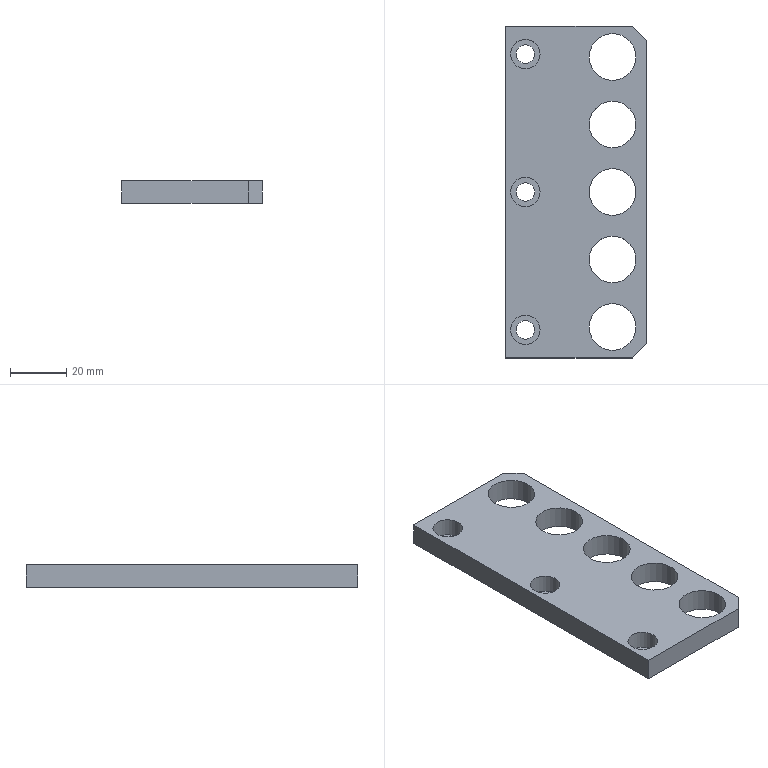Part | NX | 1 solid | 22 faces | box 50 x 118 x 8 mm | volume 36501 mm3 | cylinder 11 | plane 11 | commonest cylinder face diameters 16.6 x5 6.6 x3 10.5 x3
STEP:
#1=CARTESIAN_POINT('',(-14.7,49.,-8.));
#2=VERTEX_POINT('',#1);
#3=CARTESIAN_POINT('',(-18.,49.,-8.));
#4=DIRECTION('',(0.,0.,1.));
#5=DIRECTION('',(1.,0.,0.));
#6=AXIS2_PLACEMENT_3D('',#3,#4,#5);
#7=CIRCLE('',#6,3.3);
#8=EDGE_CURVE('',#2,#2,#7,.F.);
#9=ORIENTED_EDGE('',*,*,#8,.T.);
#10=EDGE_LOOP('',(#9));
#11=FACE_BOUND('',#10,.T.);
#12=CARTESIAN_POINT('',(-14.7,49.,-6.5));
#13=VERTEX_POINT('',#12);
#14=CARTESIAN_POINT('',(-18.,49.,-6.5));
#15=DIRECTION('',(0.,0.,1.));
#16=DIRECTION('',(1.,0.,0.));
#17=AXIS2_PLACEMENT_3D('',#14,#15,#16);
#18=CIRCLE('',#17,3.3);
#19=EDGE_CURVE('',#13,#13,#18,.F.);
#20=ORIENTED_EDGE('',*,*,#19,.F.);
#21=EDGE_LOOP('',(#20));
#22=FACE_BOUND('',#21,.T.);
#23=CARTESIAN_POINT('',(-18.,49.,-8.));
#24=DIRECTION('',(0.,0.,1.));
#25=DIRECTION('',(1.,0.,0.));
#26=AXIS2_PLACEMENT_3D('',#23,#24,#25);
#27=CYLINDRICAL_SURFACE('',#26,3.3);
#28=ADVANCED_FACE('',(#11,#22),#27,.F.);
#29=CARTESIAN_POINT('',(21.3,48.,0.));
#30=VERTEX_POINT('',#29);
#31=CARTESIAN_POINT('',(13.,48.,0.));
#32=DIRECTION('',(0.,0.,1.));
#33=DIRECTION('',(1.,0.,0.));
#34=AXIS2_PLACEMENT_3D('',#31,#32,#33);
#35=CIRCLE('',#34,8.3);
#36=EDGE_CURVE('',#30,#30,#35,.F.);
#37=ORIENTED_EDGE('',*,*,#36,.T.);
#38=EDGE_LOOP('',(#37));
#39=FACE_BOUND('',#38,.T.);
#40=CARTESIAN_POINT('',(21.3,24.,0.));
#41=VERTEX_POINT('',#40);
#42=CARTESIAN_POINT('',(13.,24.,0.));
#43=DIRECTION('',(0.,0.,1.));
#44=DIRECTION('',(1.,0.,0.));
#45=AXIS2_PLACEMENT_3D('',#42,#43,#44);
#46=CIRCLE('',#45,8.3);
#47=EDGE_CURVE('',#41,#41,#46,.F.);
#48=ORIENTED_EDGE('',*,*,#47,.T.);
#49=EDGE_LOOP('',(#48));
#50=FACE_BOUND('',#49,.T.);
#51=CARTESIAN_POINT('',(21.3,0.,0.));
#52=VERTEX_POINT('',#51);
#53=CARTESIAN_POINT('',(13.,0.,0.));
#54=DIRECTION('',(0.,0.,1.));
#55=DIRECTION('',(1.,0.,0.));
#56=AXIS2_PLACEMENT_3D('',#53,#54,#55);
#57=CIRCLE('',#56,8.3);
#58=EDGE_CURVE('',#52,#52,#57,.F.);
#59=ORIENTED_EDGE('',*,*,#58,.T.);
#60=EDGE_LOOP('',(#59));
#61=FACE_BOUND('',#60,.T.);
#62=CARTESIAN_POINT('',(21.3,-24.,0.));
#63=VERTEX_POINT('',#62);
#64=CARTESIAN_POINT('',(13.,-24.,0.));
#65=DIRECTION('',(0.,0.,1.));
#66=DIRECTION('',(1.,0.,0.));
#67=AXIS2_PLACEMENT_3D('',#64,#65,#66);
#68=CIRCLE('',#67,8.3);
#69=EDGE_CURVE('',#63,#63,#68,.F.);
#70=ORIENTED_EDGE('',*,*,#69,.T.);
#71=EDGE_LOOP('',(#70));
#72=FACE_BOUND('',#71,.T.);
#73=CARTESIAN_POINT('',(21.3,-48.,0.));
#74=VERTEX_POINT('',#73);
#75=CARTESIAN_POINT('',(13.,-48.,0.));
#76=DIRECTION('',(0.,0.,1.));
#77=DIRECTION('',(1.,0.,0.));
#78=AXIS2_PLACEMENT_3D('',#75,#76,#77);
#79=CIRCLE('',#78,8.3);
#80=EDGE_CURVE('',#74,#74,#79,.F.);
#81=ORIENTED_EDGE('',*,*,#80,.T.);
#82=EDGE_LOOP('',(#81));
#83=FACE_BOUND('',#82,.T.);
#84=CARTESIAN_POINT('',(-25.,-59.,0.));
#85=VERTEX_POINT('',#84);
#86=CARTESIAN_POINT('',(-25.,59.,0.));
#87=VERTEX_POINT('',#86);
#88=CARTESIAN_POINT('',(-25.,59.,0.));
#89=DIRECTION('',(0.,-1.,0.));
#90=VECTOR('',#89,1000.);
#91=LINE('',#88,#90);
#92=EDGE_CURVE('',#85,#87,#91,.F.);
#93=ORIENTED_EDGE('',*,*,#92,.F.);
#94=CARTESIAN_POINT('',(20.,-59.,0.));
#95=VERTEX_POINT('',#94);
#96=CARTESIAN_POINT('',(-25.,-59.,0.));
#97=DIRECTION('',(1.,0.,0.));
#98=VECTOR('',#97,1000.);
#99=LINE('',#96,#98);
#100=EDGE_CURVE('',#95,#85,#99,.F.);
#101=ORIENTED_EDGE('',*,*,#100,.F.);
#102=CARTESIAN_POINT('',(25.,-54.,0.));
#103=VERTEX_POINT('',#102);
#104=CARTESIAN_POINT('',(20.,-59.,0.));
#105=DIRECTION('',(0.7071,0.7071,0.));
#106=VECTOR('',#105,1000.);
#107=LINE('',#104,#106);
#108=EDGE_CURVE('',#103,#95,#107,.F.);
#109=ORIENTED_EDGE('',*,*,#108,.F.);
#110=CARTESIAN_POINT('',(25.,54.,0.));
#111=VERTEX_POINT('',#110);
#112=CARTESIAN_POINT('',(25.,-54.,0.));
#113=DIRECTION('',(0.,1.,0.));
#114=VECTOR('',#113,1000.);
#115=LINE('',#112,#114);
#116=EDGE_CURVE('',#111,#103,#115,.F.);
#117=ORIENTED_EDGE('',*,*,#116,.F.);
#118=CARTESIAN_POINT('',(20.,59.,0.));
#119=VERTEX_POINT('',#118);
#120=CARTESIAN_POINT('',(25.,54.,0.));
#121=DIRECTION('',(-0.7071,0.7071,0.));
#122=VECTOR('',#121,1000.);
#123=LINE('',#120,#122);
#124=EDGE_CURVE('',#119,#111,#123,.F.);
#125=ORIENTED_EDGE('',*,*,#124,.F.);
#126=CARTESIAN_POINT('',(20.,59.,0.));
#127=DIRECTION('',(-1.,0.,0.));
#128=VECTOR('',#127,1000.);
#129=LINE('',#126,#128);
#130=EDGE_CURVE('',#87,#119,#129,.F.);
#131=ORIENTED_EDGE('',*,*,#130,.F.);
#132=EDGE_LOOP('',(#93,#101,#109,#117,#125,#131));
#133=FACE_BOUND('',#132,.T.);
#134=CARTESIAN_POINT('',(-23.25,0.,0.));
#135=VERTEX_POINT('',#134);
#136=CARTESIAN_POINT('',(-18.,0.,0.));
#137=DIRECTION('',(0.,0.,-1.));
#138=DIRECTION('',(-1.,0.,0.));
#139=AXIS2_PLACEMENT_3D('',#136,#137,#138);
#140=CIRCLE('',#139,5.25);
#141=EDGE_CURVE('',#135,#135,#140,.T.);
#142=ORIENTED_EDGE('',*,*,#141,.T.);
#143=EDGE_LOOP('',(#142));
#144=FACE_BOUND('',#143,.T.);
#145=CARTESIAN_POINT('',(-23.25,-49.,0.));
#146=VERTEX_POINT('',#145);
#147=CARTESIAN_POINT('',(-18.,-49.,0.));
#148=DIRECTION('',(0.,0.,-1.));
#149=DIRECTION('',(-1.,0.,0.));
#150=AXIS2_PLACEMENT_3D('',#147,#148,#149);
#151=CIRCLE('',#150,5.25);
#152=EDGE_CURVE('',#146,#146,#151,.T.);
#153=ORIENTED_EDGE('',*,*,#152,.T.);
#154=EDGE_LOOP('',(#153));
#155=FACE_BOUND('',#154,.T.);
#156=CARTESIAN_POINT('',(-12.75,49.,0.));
#157=VERTEX_POINT('',#156);
#158=CARTESIAN_POINT('',(-18.,49.,0.));
#159=DIRECTION('',(0.,0.,1.));
#160=DIRECTION('',(1.,0.,0.));
#161=AXIS2_PLACEMENT_3D('',#158,#159,#160);
#162=CIRCLE('',#161,5.25);
#163=EDGE_CURVE('',#157,#157,#162,.T.);
#164=ORIENTED_EDGE('',*,*,#163,.F.);
#165=EDGE_LOOP('',(#164));
#166=FACE_BOUND('',#165,.T.);
#167=CARTESIAN_POINT('',(-18.,-49.,0.));
#168=DIRECTION('',(0.,0.,1.));
#169=DIRECTION('',(1.,0.,0.));
#170=AXIS2_PLACEMENT_3D('',#167,#168,#169);
#171=PLANE('',#170);
#172=ADVANCED_FACE('',(#39,#50,#61,#72,#83,#133,#144,#155,#166),#171,.T.);
#173=ORIENTED_EDGE('',*,*,#92,.T.);
#174=CARTESIAN_POINT('',(-25.,59.,-8.));
#175=VERTEX_POINT('',#174);
#176=CARTESIAN_POINT('',(-25.,59.,-8.));
#177=DIRECTION('',(0.,0.,1.));
#178=VECTOR('',#177,1000.);
#179=LINE('',#176,#178);
#180=EDGE_CURVE('',#87,#175,#179,.F.);
#181=ORIENTED_EDGE('',*,*,#180,.T.);
#182=CARTESIAN_POINT('',(-25.,-59.,-8.));
#183=VERTEX_POINT('',#182);
#184=CARTESIAN_POINT('',(-25.,59.,-8.));
#185=DIRECTION('',(0.,-1.,0.));
#186=VECTOR('',#185,1000.);
#187=LINE('',#184,#186);
#188=EDGE_CURVE('',#183,#175,#187,.F.);
#189=ORIENTED_EDGE('',*,*,#188,.F.);
#190=CARTESIAN_POINT('',(-25.,-59.,-8.));
#191=DIRECTION('',(0.,0.,1.));
#192=VECTOR('',#191,1000.);
#193=LINE('',#190,#192);
#194=EDGE_CURVE('',#85,#183,#193,.F.);
#195=ORIENTED_EDGE('',*,*,#194,.F.);
#196=EDGE_LOOP('',(#173,#181,#189,#195));
#197=FACE_BOUND('',#196,.T.);
#198=CARTESIAN_POINT('',(-25.,59.,-8.));
#199=DIRECTION('',(-1.,0.,0.));
#200=DIRECTION('',(0.,0.,1.));
#201=AXIS2_PLACEMENT_3D('',#198,#199,#200);
#202=PLANE('',#201);
#203=ADVANCED_FACE('',(#197),#202,.T.);
#204=ORIENTED_EDGE('',*,*,#100,.T.);
#205=ORIENTED_EDGE('',*,*,#194,.T.);
#206=CARTESIAN_POINT('',(20.,-59.,-8.));
#207=VERTEX_POINT('',#206);
#208=CARTESIAN_POINT('',(-25.,-59.,-8.));
#209=DIRECTION('',(1.,0.,0.));
#210=VECTOR('',#209,1000.);
#211=LINE('',#208,#210);
#212=EDGE_CURVE('',#207,#183,#211,.F.);
#213=ORIENTED_EDGE('',*,*,#212,.F.);
#214=CARTESIAN_POINT('',(20.,-59.,-8.));
#215=DIRECTION('',(0.,0.,1.));
#216=VECTOR('',#215,1000.);
#217=LINE('',#214,#216);
#218=EDGE_CURVE('',#95,#207,#217,.F.);
#219=ORIENTED_EDGE('',*,*,#218,.F.);
#220=EDGE_LOOP('',(#204,#205,#213,#219));
#221=FACE_BOUND('',#220,.T.);
#222=CARTESIAN_POINT('',(-25.,-59.,-8.));
#223=DIRECTION('',(0.,-1.,0.));
#224=DIRECTION('',(0.,0.,-1.));
#225=AXIS2_PLACEMENT_3D('',#222,#223,#224);
#226=PLANE('',#225);
#227=ADVANCED_FACE('',(#221),#226,.T.);
#228=ORIENTED_EDGE('',*,*,#108,.T.);
#229=ORIENTED_EDGE('',*,*,#218,.T.);
#230=CARTESIAN_POINT('',(25.,-54.,-8.));
#231=VERTEX_POINT('',#230);
#232=CARTESIAN_POINT('',(20.,-59.,-8.));
#233=DIRECTION('',(0.7071,0.7071,0.));
#234=VECTOR('',#233,1000.);
#235=LINE('',#232,#234);
#236=EDGE_CURVE('',#231,#207,#235,.F.);
#237=ORIENTED_EDGE('',*,*,#236,.F.);
#238=CARTESIAN_POINT('',(25.,-54.,-8.));
#239=DIRECTION('',(0.,0.,1.));
#240=VECTOR('',#239,1000.);
#241=LINE('',#238,#240);
#242=EDGE_CURVE('',#103,#231,#241,.F.);
#243=ORIENTED_EDGE('',*,*,#242,.F.);
#244=EDGE_LOOP('',(#228,#229,#237,#243));
#245=FACE_BOUND('',#244,.T.);
#246=CARTESIAN_POINT('',(20.,-59.,-8.));
#247=DIRECTION('',(0.7071,-0.7071,0.));
#248=DIRECTION('',(0.7071,0.7071,0.));
#249=AXIS2_PLACEMENT_3D('',#246,#247,#248);
#250=PLANE('',#249);
#251=ADVANCED_FACE('',(#245),#250,.T.);
#252=ORIENTED_EDGE('',*,*,#116,.T.);
#253=ORIENTED_EDGE('',*,*,#242,.T.);
#254=CARTESIAN_POINT('',(25.,54.,-8.));
#255=VERTEX_POINT('',#254);
#256=CARTESIAN_POINT('',(25.,-54.,-8.));
#257=DIRECTION('',(0.,1.,0.));
#258=VECTOR('',#257,1000.);
#259=LINE('',#256,#258);
#260=EDGE_CURVE('',#255,#231,#259,.F.);
#261=ORIENTED_EDGE('',*,*,#260,.F.);
#262=CARTESIAN_POINT('',(25.,54.,-8.));
#263=DIRECTION('',(0.,0.,1.));
#264=VECTOR('',#263,1000.);
#265=LINE('',#262,#264);
#266=EDGE_CURVE('',#111,#255,#265,.F.);
#267=ORIENTED_EDGE('',*,*,#266,.F.);
#268=EDGE_LOOP('',(#252,#253,#261,#267));
#269=FACE_BOUND('',#268,.T.);
#270=CARTESIAN_POINT('',(25.,-54.,-8.));
#271=DIRECTION('',(1.,0.,0.));
#272=DIRECTION('',(0.,0.,-1.));
#273=AXIS2_PLACEMENT_3D('',#270,#271,#272);
#274=PLANE('',#273);
#275=ADVANCED_FACE('',(#269),#274,.T.);
#276=ORIENTED_EDGE('',*,*,#124,.T.);
#277=ORIENTED_EDGE('',*,*,#266,.T.);
#278=CARTESIAN_POINT('',(20.,59.,-8.));
#279=VERTEX_POINT('',#278);
#280=CARTESIAN_POINT('',(25.,54.,-8.));
#281=DIRECTION('',(-0.7071,0.7071,0.));
#282=VECTOR('',#281,1000.);
#283=LINE('',#280,#282);
#284=EDGE_CURVE('',#279,#255,#283,.F.);
#285=ORIENTED_EDGE('',*,*,#284,.F.);
#286=CARTESIAN_POINT('',(20.,59.,-8.));
#287=DIRECTION('',(0.,0.,1.));
#288=VECTOR('',#287,1000.);
#289=LINE('',#286,#288);
#290=EDGE_CURVE('',#119,#279,#289,.F.);
#291=ORIENTED_EDGE('',*,*,#290,.F.);
#292=EDGE_LOOP('',(#276,#277,#285,#291));
#293=FACE_BOUND('',#292,.T.);
#294=CARTESIAN_POINT('',(25.,54.,-8.));
#295=DIRECTION('',(0.7071,0.7071,0.));
#296=DIRECTION('',(-0.7071,0.7071,0.));
#297=AXIS2_PLACEMENT_3D('',#294,#295,#296);
#298=PLANE('',#297);
#299=ADVANCED_FACE('',(#293),#298,.T.);
#300=CARTESIAN_POINT('',(21.3,24.,-8.));
#301=VERTEX_POINT('',#300);
#302=CARTESIAN_POINT('',(13.,24.,-8.));
#303=DIRECTION('',(0.,0.,1.));
#304=DIRECTION('',(1.,0.,0.));
#305=AXIS2_PLACEMENT_3D('',#302,#303,#304);
#306=CIRCLE('',#305,8.3);
#307=EDGE_CURVE('',#301,#301,#306,.F.);
#308=ORIENTED_EDGE('',*,*,#307,.T.);
#309=EDGE_LOOP('',(#308));
#310=FACE_BOUND('',#309,.T.);
#311=ORIENTED_EDGE('',*,*,#47,.F.);
#312=EDGE_LOOP('',(#311));
#313=FACE_BOUND('',#312,.T.);
#314=CARTESIAN_POINT('',(13.,24.,-8.));
#315=DIRECTION('',(0.,0.,1.));
#316=DIRECTION('',(1.,0.,0.));
#317=AXIS2_PLACEMENT_3D('',#314,#315,#316);
#318=CYLINDRICAL_SURFACE('',#317,8.3);
#319=ADVANCED_FACE('',(#310,#313),#318,.F.);
#320=CARTESIAN_POINT('',(21.3,0.,-8.));
#321=VERTEX_POINT('',#320);
#322=CARTESIAN_POINT('',(13.,0.,-8.));
#323=DIRECTION('',(0.,0.,1.));
#324=DIRECTION('',(1.,0.,0.));
#325=AXIS2_PLACEMENT_3D('',#322,#323,#324);
#326=CIRCLE('',#325,8.3);
#327=EDGE_CURVE('',#321,#321,#326,.F.);
#328=ORIENTED_EDGE('',*,*,#327,.T.);
#329=EDGE_LOOP('',(#328));
#330=FACE_BOUND('',#329,.T.);
#331=ORIENTED_EDGE('',*,*,#58,.F.);
#332=EDGE_LOOP('',(#331));
#333=FACE_BOUND('',#332,.T.);
#334=CARTESIAN_POINT('',(13.,0.,-8.));
#335=DIRECTION('',(0.,0.,1.));
#336=DIRECTION('',(1.,0.,0.));
#337=AXIS2_PLACEMENT_3D('',#334,#335,#336);
#338=CYLINDRICAL_SURFACE('',#337,8.3);
#339=ADVANCED_FACE('',(#330,#333),#338,.F.);
#340=CARTESIAN_POINT('',(21.3,-24.,-8.));
#341=VERTEX_POINT('',#340);
#342=CARTESIAN_POINT('',(13.,-24.,-8.));
#343=DIRECTION('',(0.,0.,1.));
#344=DIRECTION('',(1.,0.,0.));
#345=AXIS2_PLACEMENT_3D('',#342,#343,#344);
#346=CIRCLE('',#345,8.3);
#347=EDGE_CURVE('',#341,#341,#346,.F.);
#348=ORIENTED_EDGE('',*,*,#347,.T.);
#349=EDGE_LOOP('',(#348));
#350=FACE_BOUND('',#349,.T.);
#351=ORIENTED_EDGE('',*,*,#69,.F.);
#352=EDGE_LOOP('',(#351));
#353=FACE_BOUND('',#352,.T.);
#354=CARTESIAN_POINT('',(13.,-24.,-8.));
#355=DIRECTION('',(0.,0.,1.));
#356=DIRECTION('',(1.,0.,0.));
#357=AXIS2_PLACEMENT_3D('',#354,#355,#356);
#358=CYLINDRICAL_SURFACE('',#357,8.3);
#359=ADVANCED_FACE('',(#350,#353),#358,.F.);
#360=CARTESIAN_POINT('',(21.3,-48.,-8.));
#361=VERTEX_POINT('',#360);
#362=CARTESIAN_POINT('',(13.,-48.,-8.));
#363=DIRECTION('',(0.,0.,1.));
#364=DIRECTION('',(1.,0.,0.));
#365=AXIS2_PLACEMENT_3D('',#362,#363,#364);
#366=CIRCLE('',#365,8.3);
#367=EDGE_CURVE('',#361,#361,#366,.F.);
#368=ORIENTED_EDGE('',*,*,#367,.T.);
#369=EDGE_LOOP('',(#368));
#370=FACE_BOUND('',#369,.T.);
#371=ORIENTED_EDGE('',*,*,#80,.F.);
#372=EDGE_LOOP('',(#371));
#373=FACE_BOUND('',#372,.T.);
#374=CARTESIAN_POINT('',(13.,-48.,-8.));
#375=DIRECTION('',(0.,0.,1.));
#376=DIRECTION('',(1.,0.,0.));
#377=AXIS2_PLACEMENT_3D('',#374,#375,#376);
#378=CYLINDRICAL_SURFACE('',#377,8.3);
#379=ADVANCED_FACE('',(#370,#373),#378,.F.);
#380=CARTESIAN_POINT('',(-21.3,0.,-6.5));
#381=VERTEX_POINT('',#380);
#382=CARTESIAN_POINT('',(-18.,0.,-6.5));
#383=DIRECTION('',(0.,0.,-1.));
#384=DIRECTION('',(-1.,0.,0.));
#385=AXIS2_PLACEMENT_3D('',#382,#383,#384);
#386=CIRCLE('',#385,3.3);
#387=EDGE_CURVE('',#381,#381,#386,.F.);
#388=ORIENTED_EDGE('',*,*,#387,.T.);
#389=EDGE_LOOP('',(#388));
#390=FACE_BOUND('',#389,.T.);
#391=CARTESIAN_POINT('',(-14.7,0.,-8.));
#392=VERTEX_POINT('',#391);
#393=CARTESIAN_POINT('',(-18.,0.,-8.));
#394=DIRECTION('',(0.,0.,1.));
#395=DIRECTION('',(1.,0.,0.));
#396=AXIS2_PLACEMENT_3D('',#393,#394,#395);
#397=CIRCLE('',#396,3.3);
#398=EDGE_CURVE('',#392,#392,#397,.F.);
#399=ORIENTED_EDGE('',*,*,#398,.T.);
#400=EDGE_LOOP('',(#399));
#401=FACE_BOUND('',#400,.T.);
#402=CARTESIAN_POINT('',(-18.,0.,-8.));
#403=DIRECTION('',(0.,0.,1.));
#404=DIRECTION('',(1.,0.,0.));
#405=AXIS2_PLACEMENT_3D('',#402,#403,#404);
#406=CYLINDRICAL_SURFACE('',#405,3.3);
#407=ADVANCED_FACE('',(#390,#401),#406,.F.);
#408=CARTESIAN_POINT('',(-21.3,-49.,-6.5));
#409=VERTEX_POINT('',#408);
#410=CARTESIAN_POINT('',(-18.,-49.,-6.5));
#411=DIRECTION('',(0.,0.,-1.));
#412=DIRECTION('',(-1.,0.,0.));
#413=AXIS2_PLACEMENT_3D('',#410,#411,#412);
#414=CIRCLE('',#413,3.3);
#415=EDGE_CURVE('',#409,#409,#414,.F.);
#416=ORIENTED_EDGE('',*,*,#415,.T.);
#417=EDGE_LOOP('',(#416));
#418=FACE_BOUND('',#417,.T.);
#419=CARTESIAN_POINT('',(-14.7,-49.,-8.));
#420=VERTEX_POINT('',#419);
#421=CARTESIAN_POINT('',(-18.,-49.,-8.));
#422=DIRECTION('',(0.,0.,1.));
#423=DIRECTION('',(1.,0.,0.));
#424=AXIS2_PLACEMENT_3D('',#421,#422,#423);
#425=CIRCLE('',#424,3.3);
#426=EDGE_CURVE('',#420,#420,#425,.F.);
#427=ORIENTED_EDGE('',*,*,#426,.T.);
#428=EDGE_LOOP('',(#427));
#429=FACE_BOUND('',#428,.T.);
#430=CARTESIAN_POINT('',(-18.,-49.,-8.));
#431=DIRECTION('',(0.,0.,1.));
#432=DIRECTION('',(1.,0.,0.));
#433=AXIS2_PLACEMENT_3D('',#430,#431,#432);
#434=CYLINDRICAL_SURFACE('',#433,3.3);
#435=ADVANCED_FACE('',(#418,#429),#434,.F.);
#436=ORIENTED_EDGE('',*,*,#130,.T.);
#437=ORIENTED_EDGE('',*,*,#290,.T.);
#438=CARTESIAN_POINT('',(20.,59.,-8.));
#439=DIRECTION('',(-1.,0.,0.));
#440=VECTOR('',#439,1000.);
#441=LINE('',#438,#440);
#442=EDGE_CURVE('',#175,#279,#441,.F.);
#443=ORIENTED_EDGE('',*,*,#442,.F.);
#444=ORIENTED_EDGE('',*,*,#180,.F.);
#445=EDGE_LOOP('',(#436,#437,#443,#444));
#446=FACE_BOUND('',#445,.T.);
#447=CARTESIAN_POINT('',(20.,59.,-8.));
#448=DIRECTION('',(0.,1.,0.));
#449=DIRECTION('',(0.,0.,1.));
#450=AXIS2_PLACEMENT_3D('',#447,#448,#449);
#451=PLANE('',#450);
#452=ADVANCED_FACE('',(#446),#451,.T.);
#453=CARTESIAN_POINT('',(21.3,48.,-8.));
#454=VERTEX_POINT('',#453);
#455=CARTESIAN_POINT('',(13.,48.,-8.));
#456=DIRECTION('',(0.,0.,1.));
#457=DIRECTION('',(1.,0.,0.));
#458=AXIS2_PLACEMENT_3D('',#455,#456,#457);
#459=CIRCLE('',#458,8.3);
#460=EDGE_CURVE('',#454,#454,#459,.F.);
#461=ORIENTED_EDGE('',*,*,#460,.T.);
#462=EDGE_LOOP('',(#461));
#463=FACE_BOUND('',#462,.T.);
#464=ORIENTED_EDGE('',*,*,#36,.F.);
#465=EDGE_LOOP('',(#464));
#466=FACE_BOUND('',#465,.T.);
#467=CARTESIAN_POINT('',(13.,48.,-8.));
#468=DIRECTION('',(0.,0.,1.));
#469=DIRECTION('',(1.,0.,0.));
#470=AXIS2_PLACEMENT_3D('',#467,#468,#469);
#471=CYLINDRICAL_SURFACE('',#470,8.3);
#472=ADVANCED_FACE('',(#463,#466),#471,.F.);
#473=ORIENTED_EDGE('',*,*,#188,.T.);
#474=ORIENTED_EDGE('',*,*,#442,.T.);
#475=ORIENTED_EDGE('',*,*,#284,.T.);
#476=ORIENTED_EDGE('',*,*,#260,.T.);
#477=ORIENTED_EDGE('',*,*,#236,.T.);
#478=ORIENTED_EDGE('',*,*,#212,.T.);
#479=EDGE_LOOP('',(#473,#474,#475,#476,#477,#478));
#480=FACE_BOUND('',#479,.T.);
#481=ORIENTED_EDGE('',*,*,#426,.F.);
#482=EDGE_LOOP('',(#481));
#483=FACE_BOUND('',#482,.T.);
#484=ORIENTED_EDGE('',*,*,#398,.F.);
#485=EDGE_LOOP('',(#484));
#486=FACE_BOUND('',#485,.T.);
#487=ORIENTED_EDGE('',*,*,#8,.F.);
#488=EDGE_LOOP('',(#487));
#489=FACE_BOUND('',#488,.T.);
#490=ORIENTED_EDGE('',*,*,#367,.F.);
#491=EDGE_LOOP('',(#490));
#492=FACE_BOUND('',#491,.T.);
#493=ORIENTED_EDGE('',*,*,#347,.F.);
#494=EDGE_LOOP('',(#493));
#495=FACE_BOUND('',#494,.T.);
#496=ORIENTED_EDGE('',*,*,#327,.F.);
#497=EDGE_LOOP('',(#496));
#498=FACE_BOUND('',#497,.T.);
#499=ORIENTED_EDGE('',*,*,#307,.F.);
#500=EDGE_LOOP('',(#499));
#501=FACE_BOUND('',#500,.T.);
#502=ORIENTED_EDGE('',*,*,#460,.F.);
#503=EDGE_LOOP('',(#502));
#504=FACE_BOUND('',#503,.T.);
#505=CARTESIAN_POINT('',(-18.,-49.,-8.));
#506=DIRECTION('',(0.,0.,1.));
#507=DIRECTION('',(1.,0.,0.));
#508=AXIS2_PLACEMENT_3D('',#505,#506,#507);
#509=PLANE('',#508);
#510=ADVANCED_FACE('',(#480,#483,#486,#489,#492,#495,#498,#501,#504),#509,.F.);
#511=CARTESIAN_POINT('',(-23.25,0.,-6.5));
#512=VERTEX_POINT('',#511);
#513=CARTESIAN_POINT('',(-18.,0.,-6.5));
#514=DIRECTION('',(0.,0.,-1.));
#515=DIRECTION('',(-1.,0.,0.));
#516=AXIS2_PLACEMENT_3D('',#513,#514,#515);
#517=CIRCLE('',#516,5.25);
#518=EDGE_CURVE('',#512,#512,#517,.F.);
#519=ORIENTED_EDGE('',*,*,#518,.T.);
#520=EDGE_LOOP('',(#519));
#521=FACE_BOUND('',#520,.T.);
#522=ORIENTED_EDGE('',*,*,#387,.F.);
#523=EDGE_LOOP('',(#522));
#524=FACE_BOUND('',#523,.T.);
#525=CARTESIAN_POINT('',(-18.,0.,-6.5));
#526=DIRECTION('',(0.,0.,-1.));
#527=DIRECTION('',(-1.,0.,0.));
#528=AXIS2_PLACEMENT_3D('',#525,#526,#527);
#529=PLANE('',#528);
#530=ADVANCED_FACE('',(#521,#524),#529,.F.);
#531=ORIENTED_EDGE('',*,*,#518,.F.);
#532=EDGE_LOOP('',(#531));
#533=FACE_BOUND('',#532,.T.);
#534=ORIENTED_EDGE('',*,*,#141,.F.);
#535=EDGE_LOOP('',(#534));
#536=FACE_BOUND('',#535,.T.);
#537=CARTESIAN_POINT('',(-18.,0.,-6.5));
#538=DIRECTION('',(0.,0.,1.));
#539=DIRECTION('',(1.,0.,0.));
#540=AXIS2_PLACEMENT_3D('',#537,#538,#539);
#541=CYLINDRICAL_SURFACE('',#540,5.25);
#542=ADVANCED_FACE('',(#533,#536),#541,.F.);
#543=CARTESIAN_POINT('',(-23.25,-49.,-6.5));
#544=VERTEX_POINT('',#543);
#545=CARTESIAN_POINT('',(-18.,-49.,-6.5));
#546=DIRECTION('',(0.,0.,-1.));
#547=DIRECTION('',(-1.,0.,0.));
#548=AXIS2_PLACEMENT_3D('',#545,#546,#547);
#549=CIRCLE('',#548,5.25);
#550=EDGE_CURVE('',#544,#544,#549,.F.);
#551=ORIENTED_EDGE('',*,*,#550,.T.);
#552=EDGE_LOOP('',(#551));
#553=FACE_BOUND('',#552,.T.);
#554=ORIENTED_EDGE('',*,*,#415,.F.);
#555=EDGE_LOOP('',(#554));
#556=FACE_BOUND('',#555,.T.);
#557=CARTESIAN_POINT('',(-18.,-49.,-6.5));
#558=DIRECTION('',(0.,0.,-1.));
#559=DIRECTION('',(-1.,0.,0.));
#560=AXIS2_PLACEMENT_3D('',#557,#558,#559);
#561=PLANE('',#560);
#562=ADVANCED_FACE('',(#553,#556),#561,.F.);
#563=ORIENTED_EDGE('',*,*,#550,.F.);
#564=EDGE_LOOP('',(#563));
#565=FACE_BOUND('',#564,.T.);
#566=ORIENTED_EDGE('',*,*,#152,.F.);
#567=EDGE_LOOP('',(#566));
#568=FACE_BOUND('',#567,.T.);
#569=CARTESIAN_POINT('',(-18.,-49.,-6.5));
#570=DIRECTION('',(0.,0.,1.));
#571=DIRECTION('',(1.,0.,0.));
#572=AXIS2_PLACEMENT_3D('',#569,#570,#571);
#573=CYLINDRICAL_SURFACE('',#572,5.25);
#574=ADVANCED_FACE('',(#565,#568),#573,.F.);
#575=CARTESIAN_POINT('',(-12.75,49.,-6.5));
#576=VERTEX_POINT('',#575);
#577=CARTESIAN_POINT('',(-18.,49.,-6.5));
#578=DIRECTION('',(0.,0.,1.));
#579=DIRECTION('',(1.,0.,0.));
#580=AXIS2_PLACEMENT_3D('',#577,#578,#579);
#581=CIRCLE('',#580,5.25);
#582=EDGE_CURVE('',#576,#576,#581,.F.);
#583=ORIENTED_EDGE('',*,*,#582,.F.);
#584=EDGE_LOOP('',(#583));
#585=FACE_BOUND('',#584,.T.);
#586=ORIENTED_EDGE('',*,*,#19,.T.);
#587=EDGE_LOOP('',(#586));
#588=FACE_BOUND('',#587,.T.);
#589=CARTESIAN_POINT('',(-18.,49.,-6.5));
#590=DIRECTION('',(0.,0.,1.));
#591=DIRECTION('',(1.,0.,0.));
#592=AXIS2_PLACEMENT_3D('',#589,#590,#591);
#593=PLANE('',#592);
#594=ADVANCED_FACE('',(#585,#588),#593,.T.);
#595=ORIENTED_EDGE('',*,*,#582,.T.);
#596=EDGE_LOOP('',(#595));
#597=FACE_BOUND('',#596,.T.);
#598=ORIENTED_EDGE('',*,*,#163,.T.);
#599=EDGE_LOOP('',(#598));
#600=FACE_BOUND('',#599,.T.);
#601=CARTESIAN_POINT('',(-18.,49.,-6.5));
#602=DIRECTION('',(0.,0.,1.));
#603=DIRECTION('',(1.,0.,0.));
#604=AXIS2_PLACEMENT_3D('',#601,#602,#603);
#605=CYLINDRICAL_SURFACE('',#604,5.25);
#606=ADVANCED_FACE('',(#597,#600),#605,.F.);
#607=CLOSED_SHELL('',(#28,#172,#203,#227,#251,#275,#299,#319,#339,#359,#379,#407,#435,#452,#472,#510,#530,#542,#562,#574,#594,#606));
#608=MANIFOLD_SOLID_BREP('',#607);
#609=(LENGTH_UNIT()NAMED_UNIT(*)SI_UNIT(.MILLI.,.METRE.));
#610=UNCERTAINTY_MEASURE_WITH_UNIT(LENGTH_MEASURE(0.00001),#609,'','');
#611=(NAMED_UNIT(*)PLANE_ANGLE_UNIT()SI_UNIT($,.RADIAN.));
#612=(NAMED_UNIT(*)SI_UNIT($,.STERADIAN.)SOLID_ANGLE_UNIT());
#613=(GEOMETRIC_REPRESENTATION_CONTEXT(3)GLOBAL_UNCERTAINTY_ASSIGNED_CONTEXT((#610))GLOBAL_UNIT_ASSIGNED_CONTEXT((#609,#611,#612))REPRESENTATION_CONTEXT('',''));
#614=ADVANCED_BREP_SHAPE_REPRESENTATION('',(#608),#613);